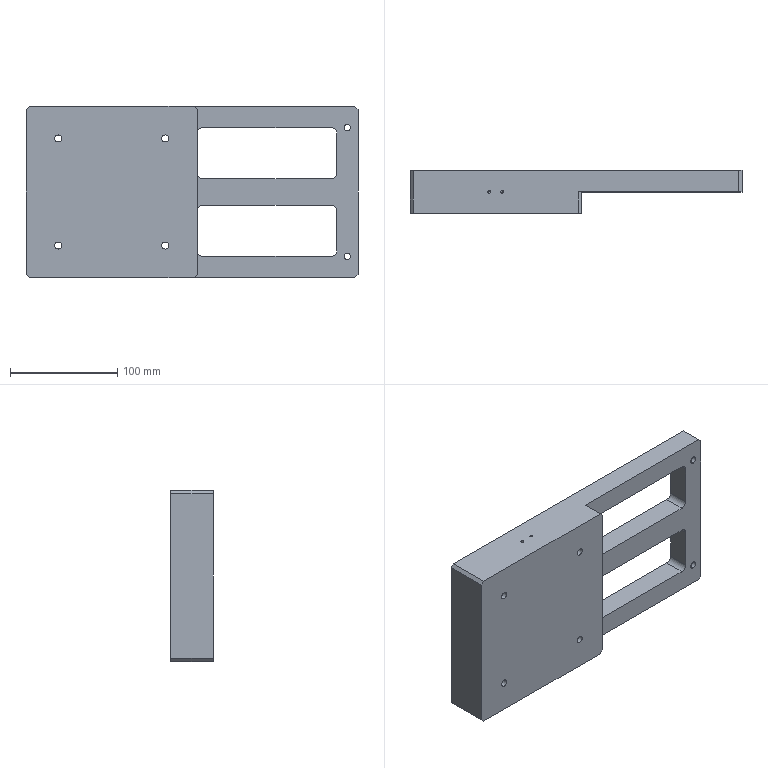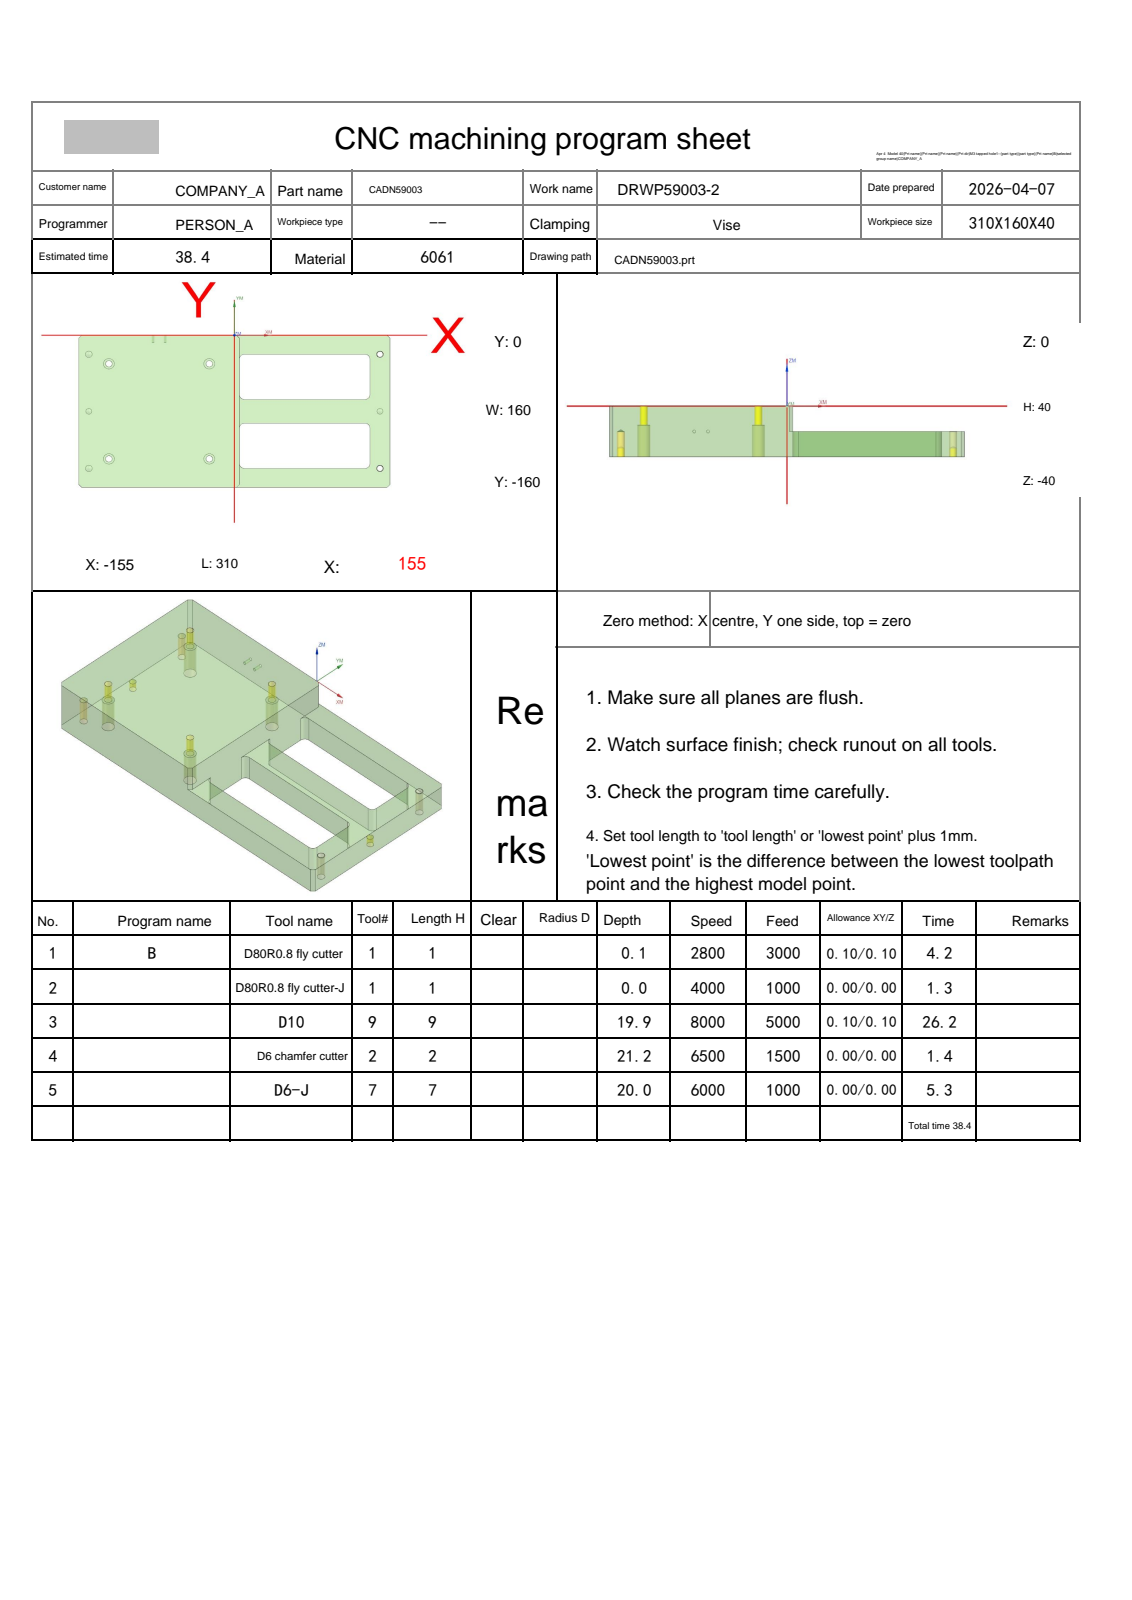NC program | NX | posted by the shop | part box 310 x 40 x 160 mm
Lines 1 to 188 of 6465:
%
O0001
(Machine time: 39.02 MIN)
(===Total Tool:4===)
(T1=D80R0.8 fly cutter D=80.  R=0.8  D-  H01 Z=-0.   )
(T9=D10     D=10.  R=0.   D-  H09 Z=-19.9 )
(T2=D6 chamfer cutter   D=6.   R=0.   D-  H02 Z=-21.2 )
(T7=D6-J    D=6.   R=0.   D7  H07 Z=-20.  )
G80 G90 G17 G49 G40
G91 G28 Z0
M01
N1 T01 M06
(D80R0.8 fly cutter  D=80. R=0.8 H=01 ce=0.10 di=0.10)
G00 G90 G54 X207.097 Y-136.097 M03 S2800
G43 H01 Z20.
M08
Z6.011
G01 Z4.011 F3000.
X195.097
X-187.101
G02 X-195.097 Y-128.101 I.004 J8.
G01 Y-91.68
G02 X-187.097 Y-83.68 I8. J0.0
G01 X187.101
G03 X195.097 Y-75.684 I-.004 J8.
G01 Y-39.263
G03 X187.097 Y-31.263 I-8. J0.0
G01 X-195.097
X-207.097
Z6.011
G00 X207.097 Y-136.097
Z5.522
G01 Z3.522
X195.097
X-187.101
G02 X-195.097 Y-128.101 I.004 J8.
G01 Y-91.68
G02 X-187.097 Y-83.68 I8. J0.0
G01 X187.101
G03 X195.097 Y-75.684 I-.004 J8.
G01 Y-39.263
G03 X187.097 Y-31.263 I-8. J0.0
G01 X-195.097
X-207.097
Z5.522
G00 X207.097 Y-136.097
Z5.033
G01 Z3.033
X195.097
X-187.101
G02 X-195.097 Y-128.101 I.004 J8.
G01 Y-91.68
G02 X-187.097 Y-83.68 I8. J0.0
G01 X187.101
G03 X195.097 Y-75.684 I-.004 J8.
G01 Y-39.263
G03 X187.097 Y-31.263 I-8. J0.0
G01 X-195.097
X-207.097
Z5.033
G00 X207.097 Y-136.097
Z4.544
G01 Z2.544
X195.097
X-187.101
G02 X-195.097 Y-128.101 I.004 J8.
G01 Y-91.68
G02 X-187.097 Y-83.68 I8. J0.0
G01 X187.101
G03 X195.097 Y-75.684 I-.004 J8.
G01 Y-39.263
G03 X187.097 Y-31.263 I-8. J0.0
G01 X-195.097
X-207.097
Z4.544
G00 Z20.
X207.097 Y-136.097
Z4.056
G01 Z2.056
X195.097
X-187.101
G02 X-195.097 Y-128.101 I.004 J8.
G01 Y-91.68
G02 X-187.097 Y-83.68 I8. J0.0
G01 X187.101
G03 X195.097 Y-75.684 I-.004 J8.
G01 Y-39.263
G03 X187.097 Y-31.263 I-8. J0.0
G01 X-195.097
X-207.097
Z4.056
G00 Z20.
X207.097 Y-136.097
Z3.567
G01 Z1.567
X195.097
X-187.101
G02 X-195.097 Y-128.101 I.004 J8.
G01 Y-91.68
G02 X-187.097 Y-83.68 I8. J0.0
G01 X187.101
G03 X195.097 Y-75.684 I-.004 J8.
G01 Y-39.263
G03 X187.097 Y-31.263 I-8. J0.0
G01 X-195.097
X-207.097
Z3.567
G00 Z20.
X207.097 Y-136.097
Z3.078
G01 Z1.078
X195.097
X-187.101
G02 X-195.097 Y-128.101 I.004 J8.
G01 Y-91.68
G02 X-187.097 Y-83.68 I8. J0.0
G01 X187.101
G03 X195.097 Y-75.684 I-.004 J8.
G01 Y-39.263
G03 X187.097 Y-31.263 I-8. J0.0
G01 X-195.097
X-207.097
Z3.078
G00 Z20.
X207.097 Y-136.097
Z2.589
G01 Z.589
X195.097
X-187.101
G02 X-195.097 Y-128.101 I.004 J8.
G01 Y-91.68
G02 X-187.097 Y-83.68 I8. J0.0
G01 X187.101
G03 X195.097 Y-75.684 I-.004 J8.
G01 Y-39.263
G03 X187.097 Y-31.263 I-8. J0.0
G01 X-195.097
X-207.097
Z2.589
G00 Z20.
X207.097 Y-136.097
Z2.1
G01 Z.1
X195.097
X-187.101
G02 X-195.097 Y-128.101 I.004 J8.
G01 Y-91.68
G02 X-187.097 Y-83.68 I8. J0.0
G01 X187.101
G03 X195.097 Y-75.684 I-.004 J8.
G01 Y-39.263
G03 X187.097 Y-31.263 I-8. J0.0
G01 X-195.097
X-207.097
Z2.1
G00 Z20.
G91 G28 Z0.0
M05
M09
G91 G28 Z0.0
M01
N2 T01 M06
(D80R0.8 fly cutter-J  D=80. R=0.8 H=01 ce=0.00 di=0.00)
G00 G90 G54 X206.999 Y-135.999 M03 S4000
G43 H01 Z20.
M08
Z2.
G01 Z0.0 F1000.
X194.999
X-187.003
G02 X-194.999 Y-128.003 I.004 J8.
G01 Y-91.68
G02 X-186.999 Y-83.68 I8. J0.0
G01 X187.003
G03 X194.999 Y-75.684 I-.004 J8.
G01 Y-38.561
G03 X187.799 Y-31.361 I-7.2 J0.0
G01 X-194.999
X-206.999
Z2.
G00 Z20.
G91 G28 Z0.0
M05
M09
G91 G28 Z0.0
M01